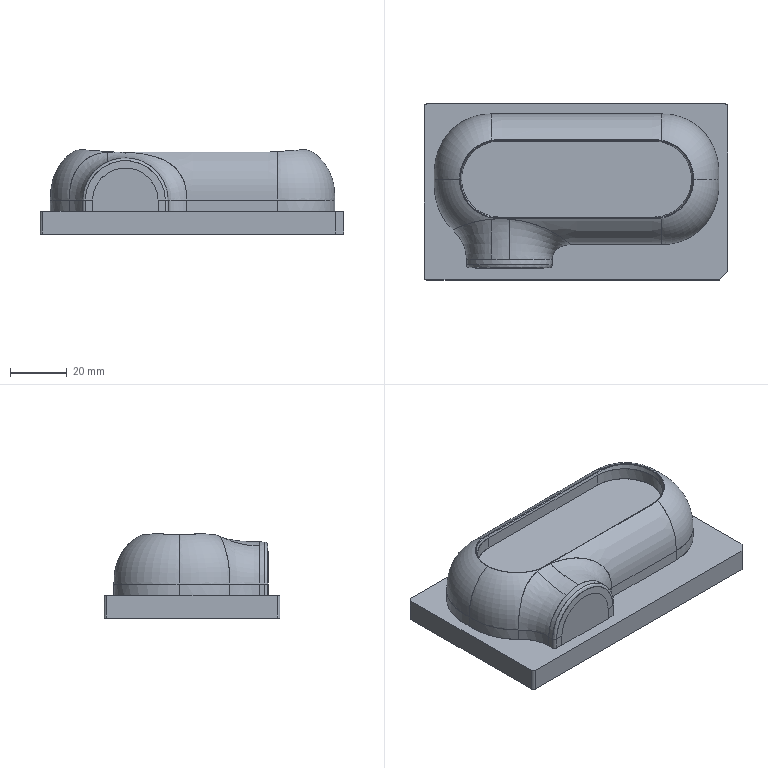CAM job | PowerMill | 3-axis milling, other | part box 107 x 62 x 29.663 mm
Tools:
number,name,type,diameter,tip_radius,length,cutting_length,overhang,flutes,holder,toolpaths_using
1,D10C_1_1_1,end_mill,10.0,0.0,60.0,,30.12,1,D42L35,4
3,D10_1_1_1,end_mill,10.0,0.0,60.0,,29.84,1,D42L35,4
17,R3_j01_1_1,ball_nosed,6.0,3.0,50.0,,20.84,1,D42L35,1
14,D4_j02_1_1,end_mill,4.0,0.0,30.0,,6.48,1,D42L35,1
13,Text_D4_1_1,taper_spherical,4.0,0.3,60.0,,21.84,1,D42L35,1
Operations:
program,toolpath,strategy,tool,tool_number,tool_diameter,tip_radius,flutes,spindle_rpm,feed_cut,surface_speed_m_min_computed,feed_per_tooth_computed,tolerance,thickness,stepover,stepdown,cut_length,cut_time_min,total_time_min,workplane
06-B01-0512-F,精公开粗01-扫面平行-D10C,raster_area_clear,D10C_1_1_1,1,10.0,0.0,1.0,8000.0,10000.0,251.33,1.25,0.03,0.32,6.0,1.0,1531.96,0.153,0.1633,
06-B01-0512-F,精公开粗01-外形偏置-D10C,offset_area_clear,D10C_1_1_1,1,10.0,0.0,1.0,8000.0,10000.0,251.33,1.25,0.03,0.32,6.0,1.0,55419.642,5.542,5.835,
06-B01-0512-F,精公开粗01-平行中光-D10C,raster,D10C_1_1_1,1,10.0,0.0,1.0,8000.0,10000.0,251.33,1.25,0.03,0.32,0.3,1.0,21885.189,2.188,2.245,
06-B01-0512-F,精公开粗01-基准台等高-D10C,constantz,D10C_1_1_1,1,10.0,0.0,1.0,8000.0,10000.0,251.33,1.25,0.03,0.07,5.0,0.4,8069.093,0.807,0.8229,
06-B01-0512-F,精公基准台01-平坦面偏置-D10,offset_area_clear,D10_1_1_1,3,10.0,0.0,1.0,8500.0,600.0,267.04,0.0706,0.005,0.42,5.0,1.0,292.14,0.487,0.5118,
06-B01-0512-F,精公基准台01-基准面偏置-D10,offset_area_clear,D10_1_1_1,3,10.0,0.0,1.0,8500.0,600.0,267.04,0.0706,0.005,0.42,5.0,1.0,536.881,0.895,0.9196,
06-B01-0512-F,精公基准台01-外形侧光-D10,profile_area_clear,D10_1_1_1,3,10.0,0.0,1.0,8500.0,600.0,267.04,0.0706,0.005,-0.03,0.08,1.0,928.554,1.548,1.703,
06-B01-0512-F,精公基准台01-基准台侧光-D10,profile_area_clear,D10_1_1_1,3,10.0,0.0,1.0,8500.0,600.0,267.04,0.0706,0.005,0.0,0.08,1.0,733.234,1.222,1.293,
06-B01-0512-F,精公精光01-浅滩和陡峭-R3,inter_constz,R3_j01_1_1,17,6.0,3.0,1.0,18000.0,2500.0,339.29,0.1389,0.005,-0.035,0.08,1.0,86109.076,34.444,35.529,
06-B01-0512-F,精公精光02-等高-D4,constantz,D4_j02_1_1,14,4.0,0.0,1.0,18000.0,2000.0,226.19,0.1111,0.005,-0.035,5.0,0.04,25975.735,12.988,13.073,
06-B01-0512-F,精公刻字01-刻字-Text_D4,pattern,Text_D4_1_1,13,4.0,0.3,1.0,15000.0,1000.0,188.5,0.0667,0.005,0.0,5.0,1.0,110.795,0.111,0.1366,